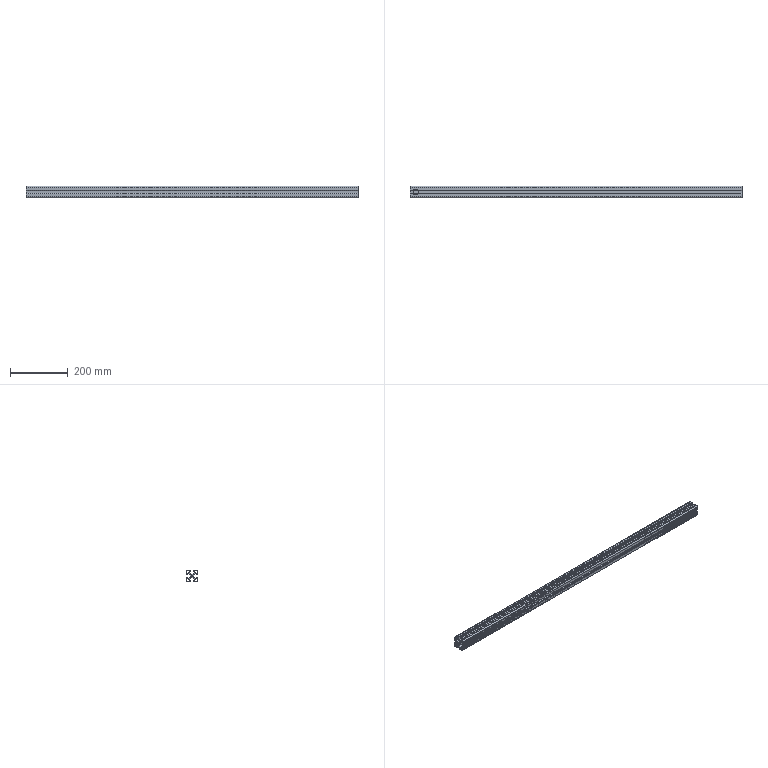Part | STEP file | MK-8-4040C-L-01 profile 4040C standard 1145mm | 1 solid | 252 faces | box 1145 x 40 x 40 mm | volume 545459 mm3 | cylinder 130 | plane 122 | commonest cylinder face diameters 0.6 x46 2 x32 4 x20 0.4 x12 19 x8 6 x4